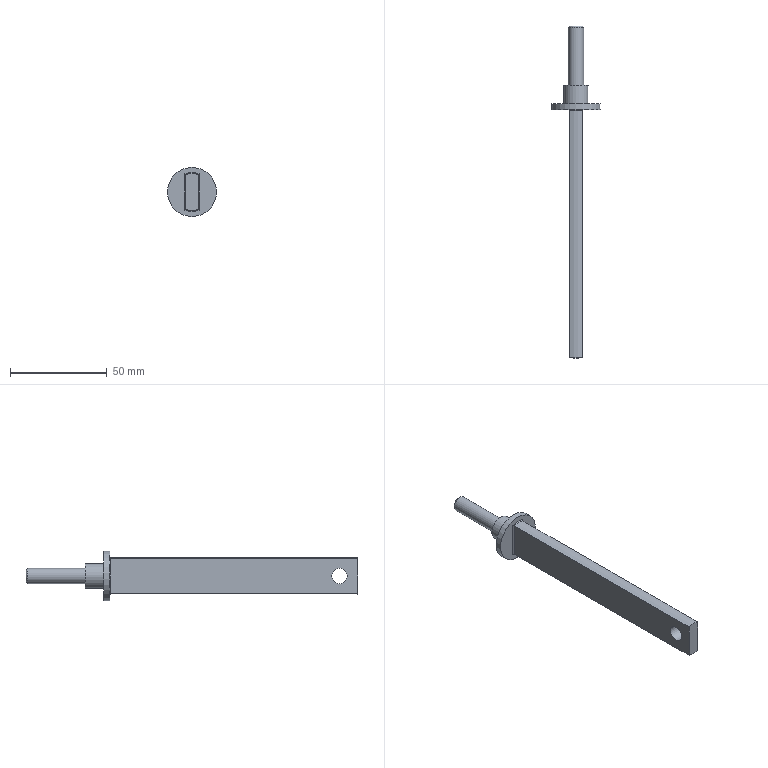Part | NX | features MG0330 trunion parts 24(stanchion group) 2 | 1 solid | 18 faces | box 25.4 x 171.609 x 25.4 mm | volume 19242 mm3 | cylinder 8 | plane 7 | torus 2 | cone 1 | commonest cylinder face diameters 1.016 x2 7.938 x2 19.05 x2 12.7 x1 25.4 x1
STEP:
#1=CARTESIAN_POINT('',(3.175,142.367,8.98));
#2=VERTEX_POINT('',#1);
#3=CARTESIAN_POINT('',(3.175,14.541,8.98));
#4=VERTEX_POINT('',#3);
#5=CARTESIAN_POINT('',(3.175,14.541,8.98));
#6=DIRECTION('',(0.,-1.,0.));
#7=VECTOR('',#6,1000.);
#8=LINE('',#5,#7);
#9=EDGE_CURVE('',#2,#4,#8,.T.);
#10=ORIENTED_EDGE('',*,*,#9,.F.);
#11=CARTESIAN_POINT('',(-3.175,142.367,8.98));
#12=VERTEX_POINT('',#11);
#13=CARTESIAN_POINT('',(0.,142.367,0.));
#14=DIRECTION('',(0.,-1.,0.));
#15=DIRECTION('',(0.,0.,-1.));
#16=AXIS2_PLACEMENT_3D('',#13,#14,#15);
#17=CIRCLE('',#16,9.525);
#18=EDGE_CURVE('',#2,#12,#17,.T.);
#19=ORIENTED_EDGE('',*,*,#18,.T.);
#20=CARTESIAN_POINT('',(-3.175,14.541,8.98));
#21=VERTEX_POINT('',#20);
#22=CARTESIAN_POINT('',(-3.175,14.541,8.98));
#23=DIRECTION('',(0.,-1.,0.));
#24=VECTOR('',#23,1000.);
#25=LINE('',#22,#24);
#26=EDGE_CURVE('',#21,#12,#25,.F.);
#27=ORIENTED_EDGE('',*,*,#26,.F.);
#28=CARTESIAN_POINT('',(0.,14.541,0.));
#29=DIRECTION('',(0.,-1.,0.));
#30=DIRECTION('',(0.,0.,-1.));
#31=AXIS2_PLACEMENT_3D('',#28,#29,#30);
#32=CIRCLE('',#31,9.525);
#33=EDGE_CURVE('',#4,#21,#32,.T.);
#34=ORIENTED_EDGE('',*,*,#33,.F.);
#35=EDGE_LOOP('',(#10,#19,#27,#34));
#36=FACE_BOUND('',#35,.T.);
#37=CARTESIAN_POINT('',(0.,14.541,0.));
#38=DIRECTION('',(0.,-1.,0.));
#39=DIRECTION('',(0.,0.,-1.));
#40=AXIS2_PLACEMENT_3D('',#37,#38,#39);
#41=CYLINDRICAL_SURFACE('',#40,9.525);
#42=ADVANCED_FACE('',(#36),#41,.T.);
#43=CARTESIAN_POINT('',(0.,146.05,-12.7));
#44=VERTEX_POINT('',#43);
#45=CARTESIAN_POINT('',(0.,146.05,0.));
#46=DIRECTION('',(0.,-1.,0.));
#47=DIRECTION('',(0.,0.,-1.));
#48=AXIS2_PLACEMENT_3D('',#45,#46,#47);
#49=CIRCLE('',#48,12.7);
#50=EDGE_CURVE('',#44,#44,#49,.T.);
#51=ORIENTED_EDGE('',*,*,#50,.T.);
#52=EDGE_LOOP('',(#51));
#53=FACE_BOUND('',#52,.T.);
#54=CARTESIAN_POINT('',(0.,142.875,-12.7));
#55=VERTEX_POINT('',#54);
#56=CARTESIAN_POINT('',(0.,142.875,0.));
#57=DIRECTION('',(0.,-1.,0.));
#58=DIRECTION('',(0.,0.,-1.));
#59=AXIS2_PLACEMENT_3D('',#56,#57,#58);
#60=CIRCLE('',#59,12.7);
#61=EDGE_CURVE('',#55,#55,#60,.T.);
#62=ORIENTED_EDGE('',*,*,#61,.F.);
#63=EDGE_LOOP('',(#62));
#64=FACE_BOUND('',#63,.T.);
#65=CARTESIAN_POINT('',(0.,14.541,0.));
#66=DIRECTION('',(0.,-1.,0.));
#67=DIRECTION('',(0.,0.,-1.));
#68=AXIS2_PLACEMENT_3D('',#65,#66,#67);
#69=CYLINDRICAL_SURFACE('',#68,12.7);
#70=ADVANCED_FACE('',(#53,#64),#69,.T.);
#71=CARTESIAN_POINT('',(0.,146.05,-6.35));
#72=VERTEX_POINT('',#71);
#73=CARTESIAN_POINT('',(0.,146.05,0.));
#74=DIRECTION('',(0.,-1.,0.));
#75=DIRECTION('',(0.,0.,-1.));
#76=AXIS2_PLACEMENT_3D('',#73,#74,#75);
#77=CIRCLE('',#76,6.35);
#78=EDGE_CURVE('',#72,#72,#77,.T.);
#79=ORIENTED_EDGE('',*,*,#78,.T.);
#80=EDGE_LOOP('',(#79));
#81=FACE_BOUND('',#80,.T.);
#82=ORIENTED_EDGE('',*,*,#50,.F.);
#83=EDGE_LOOP('',(#82));
#84=FACE_BOUND('',#83,.T.);
#85=CARTESIAN_POINT('',(12.7,146.05,0.));
#86=DIRECTION('',(0.,1.,0.));
#87=DIRECTION('',(0.,0.,1.));
#88=AXIS2_PLACEMENT_3D('',#85,#86,#87);
#89=PLANE('',#88);
#90=ADVANCED_FACE('',(#81,#84),#89,.T.);
#91=CARTESIAN_POINT('',(0.,155.575,-6.35));
#92=VERTEX_POINT('',#91);
#93=CARTESIAN_POINT('',(0.,155.575,0.));
#94=DIRECTION('',(0.,-1.,0.));
#95=DIRECTION('',(0.,0.,-1.));
#96=AXIS2_PLACEMENT_3D('',#93,#94,#95);
#97=CIRCLE('',#96,6.35);
#98=EDGE_CURVE('',#92,#92,#97,.T.);
#99=ORIENTED_EDGE('',*,*,#98,.T.);
#100=EDGE_LOOP('',(#99));
#101=FACE_BOUND('',#100,.T.);
#102=ORIENTED_EDGE('',*,*,#78,.F.);
#103=EDGE_LOOP('',(#102));
#104=FACE_BOUND('',#103,.T.);
#105=CARTESIAN_POINT('',(0.,14.541,0.));
#106=DIRECTION('',(0.,-1.,0.));
#107=DIRECTION('',(0.,0.,-1.));
#108=AXIS2_PLACEMENT_3D('',#105,#106,#107);
#109=CYLINDRICAL_SURFACE('',#108,6.35);
#110=ADVANCED_FACE('',(#101,#104),#109,.T.);
#111=CARTESIAN_POINT('',(0.,155.575,-3.969));
#112=VERTEX_POINT('',#111);
#113=CARTESIAN_POINT('',(0.,155.575,0.));
#114=DIRECTION('',(0.,-1.,0.));
#115=DIRECTION('',(0.,0.,-1.));
#116=AXIS2_PLACEMENT_3D('',#113,#114,#115);
#117=CIRCLE('',#116,3.969);
#118=EDGE_CURVE('',#112,#112,#117,.T.);
#119=ORIENTED_EDGE('',*,*,#118,.T.);
#120=EDGE_LOOP('',(#119));
#121=FACE_BOUND('',#120,.T.);
#122=ORIENTED_EDGE('',*,*,#98,.F.);
#123=EDGE_LOOP('',(#122));
#124=FACE_BOUND('',#123,.T.);
#125=CARTESIAN_POINT('',(6.35,155.575,0.));
#126=DIRECTION('',(0.,1.,0.));
#127=DIRECTION('',(0.,0.,1.));
#128=AXIS2_PLACEMENT_3D('',#125,#126,#127);
#129=PLANE('',#128);
#130=ADVANCED_FACE('',(#121,#124),#129,.T.);
#131=CARTESIAN_POINT('',(0.,185.388,3.969));
#132=VERTEX_POINT('',#131);
#133=CARTESIAN_POINT('',(0.,185.388,0.));
#134=DIRECTION('',(0.,1.,0.));
#135=DIRECTION('',(0.,0.,1.));
#136=AXIS2_PLACEMENT_3D('',#133,#134,#135);
#137=CIRCLE('',#136,3.969);
#138=EDGE_CURVE('',#132,#132,#137,.F.);
#139=ORIENTED_EDGE('',*,*,#138,.T.);
#140=EDGE_LOOP('',(#139));
#141=FACE_BOUND('',#140,.T.);
#142=ORIENTED_EDGE('',*,*,#118,.F.);
#143=EDGE_LOOP('',(#142));
#144=FACE_BOUND('',#143,.T.);
#145=CARTESIAN_POINT('',(0.,14.541,0.));
#146=DIRECTION('',(0.,-1.,0.));
#147=DIRECTION('',(0.,0.,-1.));
#148=AXIS2_PLACEMENT_3D('',#145,#146,#147);
#149=CYLINDRICAL_SURFACE('',#148,3.969);
#150=ADVANCED_FACE('',(#141,#144),#149,.T.);
#151=CARTESIAN_POINT('',(0.,186.15,3.207));
#152=VERTEX_POINT('',#151);
#153=CARTESIAN_POINT('',(0.,186.15,0.));
#154=DIRECTION('',(0.,1.,0.));
#155=DIRECTION('',(0.,0.,1.));
#156=AXIS2_PLACEMENT_3D('',#153,#154,#155);
#157=CIRCLE('',#156,3.207);
#158=EDGE_CURVE('',#152,#152,#157,.T.);
#159=ORIENTED_EDGE('',*,*,#158,.T.);
#160=EDGE_LOOP('',(#159));
#161=FACE_BOUND('',#160,.T.);
#162=CARTESIAN_POINT('',(3.969,186.15,0.));
#163=DIRECTION('',(0.,1.,0.));
#164=DIRECTION('',(0.,0.,1.));
#165=AXIS2_PLACEMENT_3D('',#162,#163,#164);
#166=PLANE('',#165);
#167=ADVANCED_FACE('',(#161),#166,.T.);
#168=CARTESIAN_POINT('',(-3.175,14.541,-8.98));
#169=VERTEX_POINT('',#168);
#170=CARTESIAN_POINT('',(-3.175,14.541,-14.287));
#171=DIRECTION('',(0.,0.,1.));
#172=VECTOR('',#171,1000.);
#173=LINE('',#170,#172);
#174=EDGE_CURVE('',#169,#21,#173,.T.);
#175=ORIENTED_EDGE('',*,*,#174,.F.);
#176=CARTESIAN_POINT('',(3.175,14.541,-8.98));
#177=VERTEX_POINT('',#176);
#178=CARTESIAN_POINT('',(0.,14.541,0.));
#179=DIRECTION('',(0.,-1.,0.));
#180=DIRECTION('',(0.,0.,-1.));
#181=AXIS2_PLACEMENT_3D('',#178,#179,#180);
#182=CIRCLE('',#181,9.525);
#183=EDGE_CURVE('',#169,#177,#182,.T.);
#184=ORIENTED_EDGE('',*,*,#183,.T.);
#185=CARTESIAN_POINT('',(3.175,14.541,-14.287));
#186=DIRECTION('',(0.,0.,1.));
#187=VECTOR('',#186,1000.);
#188=LINE('',#185,#187);
#189=EDGE_CURVE('',#177,#4,#188,.T.);
#190=ORIENTED_EDGE('',*,*,#189,.T.);
#191=ORIENTED_EDGE('',*,*,#33,.T.);
#192=EDGE_LOOP('',(#175,#184,#190,#191));
#193=FACE_BOUND('',#192,.T.);
#194=CARTESIAN_POINT('',(0.,14.541,0.));
#195=DIRECTION('',(0.,-1.,0.));
#196=DIRECTION('',(0.,0.,-1.));
#197=AXIS2_PLACEMENT_3D('',#194,#195,#196);
#198=PLANE('',#197);
#199=ADVANCED_FACE('',(#193),#198,.T.);
#200=CARTESIAN_POINT('',(-3.175,142.367,-8.98));
#201=VERTEX_POINT('',#200);
#202=CARTESIAN_POINT('',(-3.175,14.541,-8.98));
#203=DIRECTION('',(0.,-1.,0.));
#204=VECTOR('',#203,1000.);
#205=LINE('',#202,#204);
#206=EDGE_CURVE('',#201,#169,#205,.T.);
#207=ORIENTED_EDGE('',*,*,#206,.F.);
#208=CARTESIAN_POINT('',(3.175,142.367,-8.98));
#209=VERTEX_POINT('',#208);
#210=CARTESIAN_POINT('',(0.,142.367,0.));
#211=DIRECTION('',(0.,-1.,0.));
#212=DIRECTION('',(0.,0.,-1.));
#213=AXIS2_PLACEMENT_3D('',#210,#211,#212);
#214=CIRCLE('',#213,9.525);
#215=EDGE_CURVE('',#201,#209,#214,.T.);
#216=ORIENTED_EDGE('',*,*,#215,.T.);
#217=CARTESIAN_POINT('',(3.175,14.541,-8.98));
#218=DIRECTION('',(0.,-1.,0.));
#219=VECTOR('',#218,1000.);
#220=LINE('',#217,#219);
#221=EDGE_CURVE('',#177,#209,#220,.F.);
#222=ORIENTED_EDGE('',*,*,#221,.F.);
#223=ORIENTED_EDGE('',*,*,#183,.F.);
#224=EDGE_LOOP('',(#207,#216,#222,#223));
#225=FACE_BOUND('',#224,.T.);
#226=CARTESIAN_POINT('',(0.,14.541,0.));
#227=DIRECTION('',(0.,-1.,0.));
#228=DIRECTION('',(0.,0.,-1.));
#229=AXIS2_PLACEMENT_3D('',#226,#227,#228);
#230=CYLINDRICAL_SURFACE('',#229,9.525);
#231=ADVANCED_FACE('',(#225),#230,.T.);
#232=CARTESIAN_POINT('',(-3.683,142.875,9.333));
#233=VERTEX_POINT('',#232);
#234=CARTESIAN_POINT('',(3.683,142.875,9.333));
#235=VERTEX_POINT('',#234);
#236=CARTESIAN_POINT('',(0.,142.875,0.));
#237=DIRECTION('',(0.,-1.,0.));
#238=DIRECTION('',(0.,0.,-1.));
#239=AXIS2_PLACEMENT_3D('',#236,#237,#238);
#240=CIRCLE('',#239,10.033);
#241=EDGE_CURVE('',#233,#235,#240,.F.);
#242=ORIENTED_EDGE('',*,*,#241,.T.);
#243=CARTESIAN_POINT('',(3.683,142.875,-9.333));
#244=VERTEX_POINT('',#243);
#245=CARTESIAN_POINT('',(3.683,142.875,0.));
#246=DIRECTION('',(0.,0.,1.));
#247=VECTOR('',#246,1000.);
#248=LINE('',#245,#247);
#249=EDGE_CURVE('',#235,#244,#248,.F.);
#250=ORIENTED_EDGE('',*,*,#249,.T.);
#251=CARTESIAN_POINT('',(-3.683,142.875,-9.333));
#252=VERTEX_POINT('',#251);
#253=CARTESIAN_POINT('',(0.,142.875,0.));
#254=DIRECTION('',(0.,-1.,0.));
#255=DIRECTION('',(0.,0.,-1.));
#256=AXIS2_PLACEMENT_3D('',#253,#254,#255);
#257=CIRCLE('',#256,10.033);
#258=EDGE_CURVE('',#244,#252,#257,.F.);
#259=ORIENTED_EDGE('',*,*,#258,.T.);
#260=CARTESIAN_POINT('',(-3.683,142.875,0.));
#261=DIRECTION('',(0.,0.,1.));
#262=VECTOR('',#261,1000.);
#263=LINE('',#260,#262);
#264=EDGE_CURVE('',#252,#233,#263,.T.);
#265=ORIENTED_EDGE('',*,*,#264,.T.);
#266=EDGE_LOOP('',(#242,#250,#259,#265));
#267=FACE_BOUND('',#266,.T.);
#268=ORIENTED_EDGE('',*,*,#61,.T.);
#269=EDGE_LOOP('',(#268));
#270=FACE_BOUND('',#269,.T.);
#271=CARTESIAN_POINT('',(9.525,142.875,0.));
#272=DIRECTION('',(0.,-1.,0.));
#273=DIRECTION('',(0.,0.,-1.));
#274=AXIS2_PLACEMENT_3D('',#271,#272,#273);
#275=PLANE('',#274);
#276=ADVANCED_FACE('',(#267,#270),#275,.T.);
#277=ORIENTED_EDGE('',*,*,#158,.F.);
#278=EDGE_LOOP('',(#277));
#279=FACE_BOUND('',#278,.T.);
#280=ORIENTED_EDGE('',*,*,#138,.F.);
#281=EDGE_LOOP('',(#280));
#282=FACE_BOUND('',#281,.T.);
#283=CARTESIAN_POINT('',(0.,185.388,0.));
#284=DIRECTION('',(0.,-1.,0.));
#285=DIRECTION('',(0.,0.,-1.));
#286=AXIS2_PLACEMENT_3D('',#283,#284,#285);
#287=CONICAL_SURFACE('',#286,3.969,0.7854);
#288=ADVANCED_FACE('',(#279,#282),#287,.T.);
#289=CARTESIAN_POINT('',(3.175,24.067,3.969));
#290=VERTEX_POINT('',#289);
#291=CARTESIAN_POINT('',(3.175,24.067,0.));
#292=DIRECTION('',(-1.,0.,0.));
#293=DIRECTION('',(0.,0.,1.));
#294=AXIS2_PLACEMENT_3D('',#291,#292,#293);
#295=CIRCLE('',#294,3.969);
#296=EDGE_CURVE('',#290,#290,#295,.T.);
#297=ORIENTED_EDGE('',*,*,#296,.T.);
#298=EDGE_LOOP('',(#297));
#299=FACE_BOUND('',#298,.T.);
#300=ORIENTED_EDGE('',*,*,#221,.T.);
#301=CARTESIAN_POINT('',(3.175,142.367,-14.287));
#302=DIRECTION('',(0.,0.,1.));
#303=VECTOR('',#302,1000.);
#304=LINE('',#301,#303);
#305=EDGE_CURVE('',#209,#2,#304,.T.);
#306=ORIENTED_EDGE('',*,*,#305,.T.);
#307=ORIENTED_EDGE('',*,*,#9,.T.);
#308=ORIENTED_EDGE('',*,*,#189,.F.);
#309=EDGE_LOOP('',(#300,#306,#307,#308));
#310=FACE_BOUND('',#309,.T.);
#311=CARTESIAN_POINT('',(3.175,14.541,-14.287));
#312=DIRECTION('',(-1.,0.,0.));
#313=DIRECTION('',(0.,0.,1.));
#314=AXIS2_PLACEMENT_3D('',#311,#312,#313);
#315=PLANE('',#314);
#316=ADVANCED_FACE('',(#299,#310),#315,.F.);
#317=CARTESIAN_POINT('',(-3.175,24.067,-3.969));
#318=VERTEX_POINT('',#317);
#319=CARTESIAN_POINT('',(-3.175,24.067,0.));
#320=DIRECTION('',(1.,0.,0.));
#321=DIRECTION('',(0.,0.,-1.));
#322=AXIS2_PLACEMENT_3D('',#319,#320,#321);
#323=CIRCLE('',#322,3.969);
#324=EDGE_CURVE('',#318,#318,#323,.T.);
#325=ORIENTED_EDGE('',*,*,#324,.T.);
#326=EDGE_LOOP('',(#325));
#327=FACE_BOUND('',#326,.T.);
#328=ORIENTED_EDGE('',*,*,#26,.T.);
#329=CARTESIAN_POINT('',(-3.175,142.367,-14.287));
#330=DIRECTION('',(0.,0.,1.));
#331=VECTOR('',#330,1000.);
#332=LINE('',#329,#331);
#333=EDGE_CURVE('',#12,#201,#332,.F.);
#334=ORIENTED_EDGE('',*,*,#333,.T.);
#335=ORIENTED_EDGE('',*,*,#206,.T.);
#336=ORIENTED_EDGE('',*,*,#174,.T.);
#337=EDGE_LOOP('',(#328,#334,#335,#336));
#338=FACE_BOUND('',#337,.T.);
#339=CARTESIAN_POINT('',(-3.175,14.541,-14.287));
#340=DIRECTION('',(1.,0.,0.));
#341=DIRECTION('',(0.,0.,-1.));
#342=AXIS2_PLACEMENT_3D('',#339,#340,#341);
#343=PLANE('',#342);
#344=ADVANCED_FACE('',(#327,#338),#343,.F.);
#345=ORIENTED_EDGE('',*,*,#324,.F.);
#346=EDGE_LOOP('',(#345));
#347=FACE_BOUND('',#346,.T.);
#348=ORIENTED_EDGE('',*,*,#296,.F.);
#349=EDGE_LOOP('',(#348));
#350=FACE_BOUND('',#349,.T.);
#351=CARTESIAN_POINT('',(-12.7,24.067,0.));
#352=DIRECTION('',(1.,0.,0.));
#353=DIRECTION('',(0.,0.,-1.));
#354=AXIS2_PLACEMENT_3D('',#351,#352,#353);
#355=CYLINDRICAL_SURFACE('',#354,3.969);
#356=ADVANCED_FACE('',(#347,#350),#355,.F.);
#357=CARTESIAN_POINT('',(3.175,142.367,8.98));
#358=CARTESIAN_POINT('',(3.175,142.666,8.98));
#359=CARTESIAN_POINT('',(3.44,142.875,9.167));
#360=CARTESIAN_POINT('',(3.683,142.875,9.333));
#361=B_SPLINE_CURVE_WITH_KNOTS('',3,(#357,#358,#359,#360),.UNSPECIFIED.,.F.,.F.,(4,4),(0.,0.0008819),.UNSPECIFIED.);
#362=EDGE_CURVE('',#235,#2,#361,.F.);
#363=ORIENTED_EDGE('',*,*,#362,.F.);
#364=ORIENTED_EDGE('',*,*,#241,.F.);
#365=CARTESIAN_POINT('',(-3.175,142.367,8.98));
#366=CARTESIAN_POINT('',(-3.175,142.666,8.98));
#367=CARTESIAN_POINT('',(-3.44,142.875,9.167));
#368=CARTESIAN_POINT('',(-3.683,142.875,9.333));
#369=B_SPLINE_CURVE_WITH_KNOTS('',3,(#365,#366,#367,#368),.UNSPECIFIED.,.F.,.F.,(4,4),(0.,0.0008819),.UNSPECIFIED.);
#370=EDGE_CURVE('',#12,#233,#369,.T.);
#371=ORIENTED_EDGE('',*,*,#370,.F.);
#372=ORIENTED_EDGE('',*,*,#18,.F.);
#373=EDGE_LOOP('',(#363,#364,#371,#372));
#374=FACE_BOUND('',#373,.T.);
#375=CARTESIAN_POINT('',(0.,142.367,0.));
#376=DIRECTION('',(0.,-1.,0.));
#377=DIRECTION('',(0.,0.,-1.));
#378=AXIS2_PLACEMENT_3D('',#375,#376,#377);
#379=TOROIDAL_SURFACE('',#378,10.033,0.508);
#380=ADVANCED_FACE('',(#374),#379,.F.);
#381=ORIENTED_EDGE('',*,*,#370,.T.);
#382=ORIENTED_EDGE('',*,*,#264,.F.);
#383=CARTESIAN_POINT('',(-3.175,142.367,-8.98));
#384=CARTESIAN_POINT('',(-3.175,142.666,-8.98));
#385=CARTESIAN_POINT('',(-3.44,142.875,-9.167));
#386=CARTESIAN_POINT('',(-3.683,142.875,-9.333));
#387=B_SPLINE_CURVE_WITH_KNOTS('',3,(#383,#384,#385,#386),.UNSPECIFIED.,.F.,.F.,(4,4),(0.,0.0008819),.UNSPECIFIED.);
#388=EDGE_CURVE('',#201,#252,#387,.T.);
#389=ORIENTED_EDGE('',*,*,#388,.F.);
#390=ORIENTED_EDGE('',*,*,#333,.F.);
#391=EDGE_LOOP('',(#381,#382,#389,#390));
#392=FACE_BOUND('',#391,.T.);
#393=CARTESIAN_POINT('',(-3.683,142.367,0.));
#394=DIRECTION('',(0.,0.,1.));
#395=DIRECTION('',(1.,0.,0.));
#396=AXIS2_PLACEMENT_3D('',#393,#394,#395);
#397=CYLINDRICAL_SURFACE('',#396,0.508);
#398=ADVANCED_FACE('',(#392),#397,.F.);
#399=ORIENTED_EDGE('',*,*,#362,.T.);
#400=ORIENTED_EDGE('',*,*,#305,.F.);
#401=CARTESIAN_POINT('',(3.175,142.367,-8.98));
#402=CARTESIAN_POINT('',(3.175,142.666,-8.98));
#403=CARTESIAN_POINT('',(3.44,142.875,-9.167));
#404=CARTESIAN_POINT('',(3.683,142.875,-9.333));
#405=B_SPLINE_CURVE_WITH_KNOTS('',3,(#401,#402,#403,#404),.UNSPECIFIED.,.F.,.F.,(4,4),(0.,0.0008819),.UNSPECIFIED.);
#406=EDGE_CURVE('',#244,#209,#405,.F.);
#407=ORIENTED_EDGE('',*,*,#406,.F.);
#408=ORIENTED_EDGE('',*,*,#249,.F.);
#409=EDGE_LOOP('',(#399,#400,#407,#408));
#410=FACE_BOUND('',#409,.T.);
#411=CARTESIAN_POINT('',(3.683,142.367,-14.287));
#412=DIRECTION('',(0.,0.,1.));
#413=DIRECTION('',(1.,0.,0.));
#414=AXIS2_PLACEMENT_3D('',#411,#412,#413);
#415=CYLINDRICAL_SURFACE('',#414,0.508);
#416=ADVANCED_FACE('',(#410),#415,.F.);
#417=ORIENTED_EDGE('',*,*,#388,.T.);
#418=ORIENTED_EDGE('',*,*,#258,.F.);
#419=ORIENTED_EDGE('',*,*,#406,.T.);
#420=ORIENTED_EDGE('',*,*,#215,.F.);
#421=EDGE_LOOP('',(#417,#418,#419,#420));
#422=FACE_BOUND('',#421,.T.);
#423=CARTESIAN_POINT('',(0.,142.367,0.));
#424=DIRECTION('',(0.,-1.,0.));
#425=DIRECTION('',(0.,0.,-1.));
#426=AXIS2_PLACEMENT_3D('',#423,#424,#425);
#427=TOROIDAL_SURFACE('',#426,10.033,0.508);
#428=ADVANCED_FACE('',(#422),#427,.F.);
#429=CLOSED_SHELL('',(#42,#70,#90,#110,#130,#150,#167,#199,#231,#276,#288,#316,#344,#356,#380,#398,#416,#428));
#430=MANIFOLD_SOLID_BREP('',#429);
#431=(LENGTH_UNIT()NAMED_UNIT(*)SI_UNIT(.MILLI.,.METRE.));
#432=UNCERTAINTY_MEASURE_WITH_UNIT(LENGTH_MEASURE(0.0508),#431,'','');
#433=(NAMED_UNIT(*)PLANE_ANGLE_UNIT()SI_UNIT($,.RADIAN.));
#434=(NAMED_UNIT(*)SI_UNIT($,.STERADIAN.)SOLID_ANGLE_UNIT());
#435=(GEOMETRIC_REPRESENTATION_CONTEXT(3)GLOBAL_UNCERTAINTY_ASSIGNED_CONTEXT((#432))GLOBAL_UNIT_ASSIGNED_CONTEXT((#431,#433,#434))REPRESENTATION_CONTEXT('',''));
#436=ADVANCED_BREP_SHAPE_REPRESENTATION('',(#430),#435);